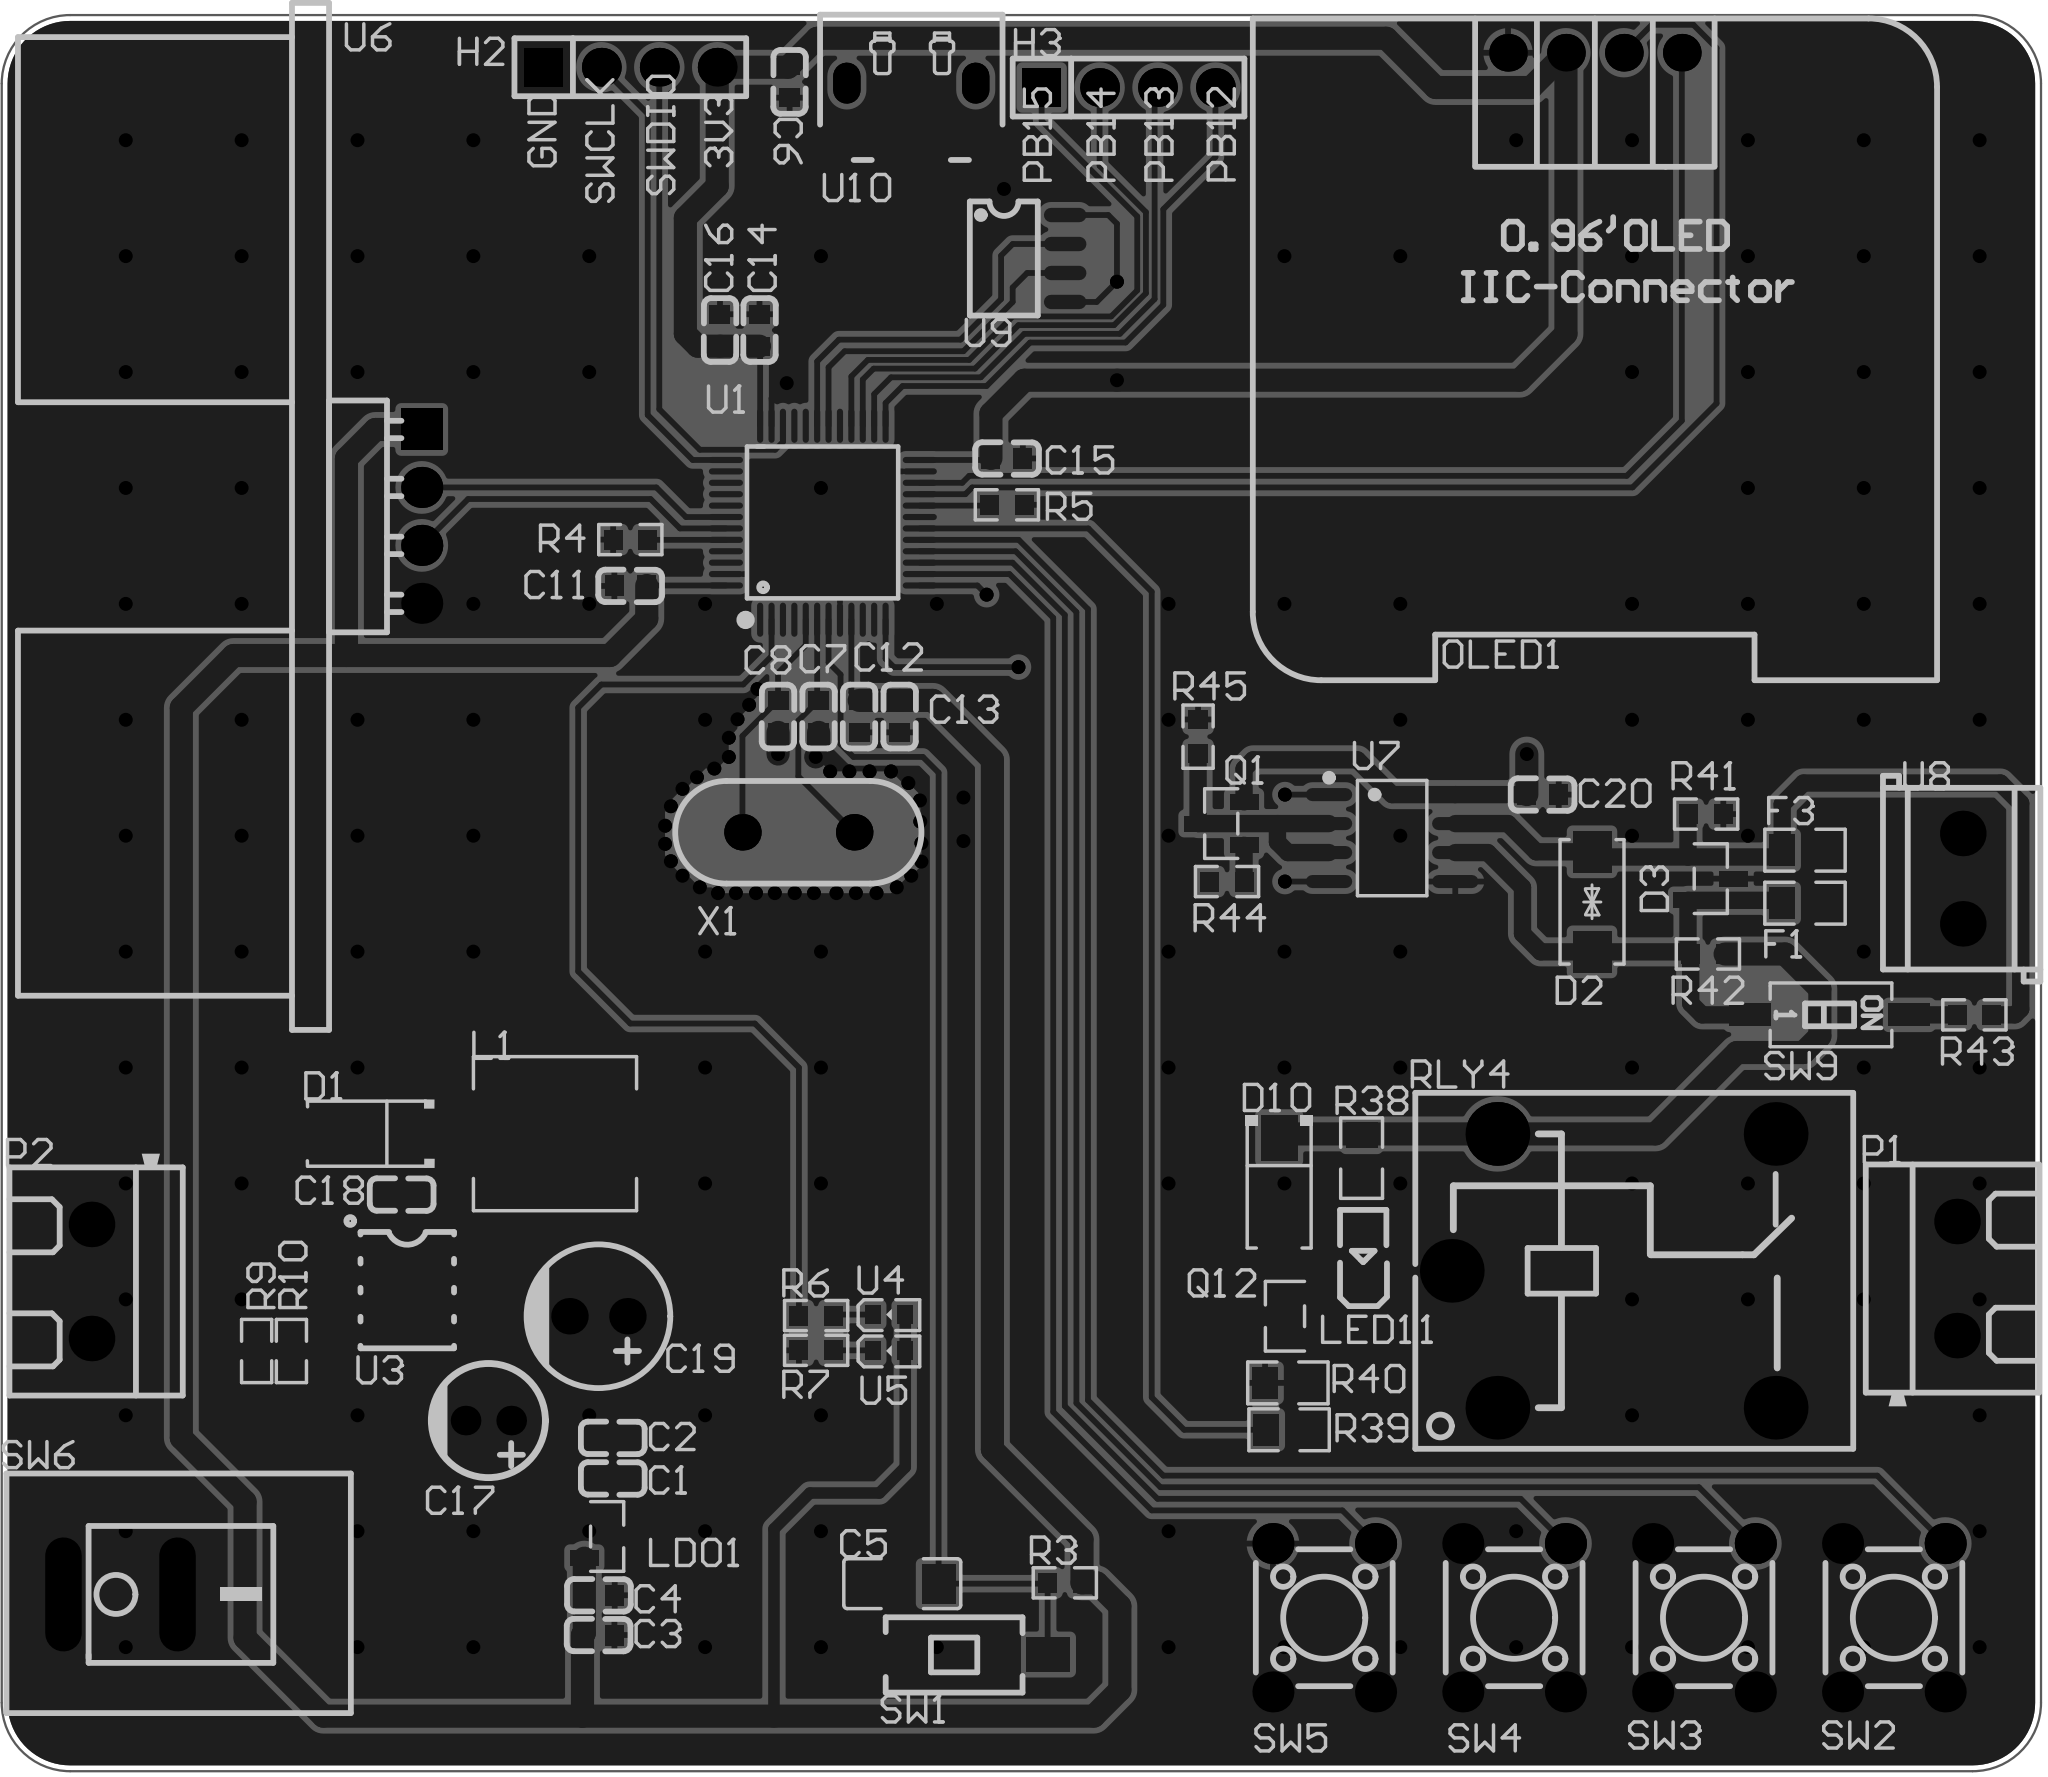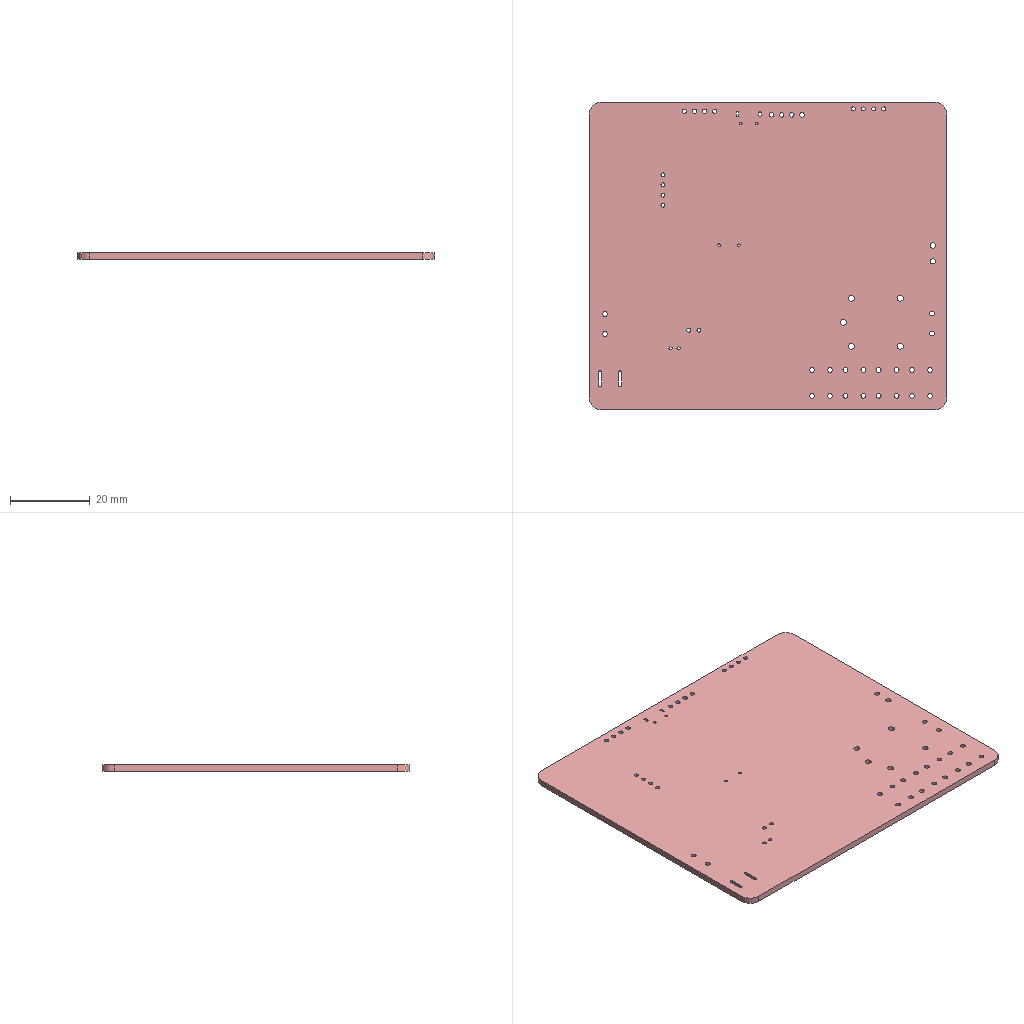Circuit board layout | Altium Designer | box 89.4 x 77 x 1.6 mm
Layer stack:
# Altium Designer layer stack of  (unit mm; dielectric type: 0 none, 1 core, 2 prepreg, 3 surface material)
index,name,kind,layer,copper_thickness_mm,dielectric_type,dielectric_thickness_mm,dielectric_material,dielectric_constant
0,Top Paste Mask Layer,other,,,,,,
1,Top Silkscreen Layer,other,,,,,,
2,Top Solder Mask Layer,dielectric,,,3,0.01,,3.3
3,Top Layer,copper,Top Layer,0.035,,,,
4,Dielectric1,dielectric,,,3,1.51,FR4,4.5
5,Bottom Layer,copper,Bottom Layer,0.035,,,,
6,Bottom Solder Mask Layer,dielectric,,,3,0.01,,3.3
7,Bottom Silkscreen Layer,other,,,,,,
8,Bottom Paste Mask Layer,other,,,,,,
# drill layer pairs: low layer,high layer
drill_pair,Top Layer,Bottom Layer
Part placement:
Designator,Comment,Layer,Footprint,Center-X(mm),Center-Y(mm),Rotation
C1,10uF,TopLayer,C0603,111.252,94.742,0
C2,100nF,TopLayer,C0603,111.252,96.52,0
C3,100nF,TopLayer,C0603,110.617,87.884,180
C4,10uF,TopLayer,C0603,110.63,89.626,180
C5,100uF,TopLayer,C1206,123.938,90.134,0
C6,100nF,TopLayer,C0603,118.999,155.956,90
C7,20pF,TopLayer,C0603,120.269,128.143,90
C8,20pF,TopLayer,C0603,118.491,128.143,90
C11,100nF,TopLayer,C0603,112.014,133.858,0
C12,100nF,TopLayer,C0603,122.047,128.143,90
C13,100nF,TopLayer,C0603,123.825,128.143,90
C14,100nF,TopLayer,C0603,117.678,145.067,270
C15,100nF,TopLayer,C0603,128.524,139.446,180
C16,4.7nF,TopLayer,C0603,115.946,145.067,270
C17,10uF,TopLayer,CAP-TH_BD5.0-P2.00-D0.8-FD,105.791,97.282,180
C18,10nF,TopLayer,C0603,101.981,107.188,180
C19,220uF,TopLayer,CAP-TH_BD6.3-P2.50-D1.0-FD,110.617,101.854,180
C20,100nF,TopLayer,C0603,152.019,124.714,0
D1,B340A,TopLayer,SMA_L4.3-W2.6-LS5.1-RD,100.457,109.855,180
D2,SMAJ7.0CA,TopLayer,SMA_L4.5-W2.7-LS5.1-BI,154.178,120.015,270
D3,SM712,TopLayer,SOT-23-3_L2.9-W1.3-P1.90-LS2.4-BR,159.385,121.031,180
D10,1N4007,TopLayer,SMA_L4.3-W2.5-LS5.0-RD,140.462,107.569,270
F1,0R,TopLayer,R0805,163.516,119.956,0
F3,0R,TopLayer,R0805,163.516,122.279,0
H2,,TopLayer,HDR-TH_4P-P2.54-V-M,112.014,156.591,0
L1,15uH,TopLayer,IND-SMD_L7.0-W6.6_FXL0630,108.712,109.855,0
LDO1,SC662K-3.3V,TopLayer,SOT-23-3_L2.9-W1.3-P1.90-LS2.4-BR,110.998,92.202,180
LED11,NCD0805R1,TopLayer,LED0805-R-RD,144.145,104.521,90
OLED1,,TopLayer,0.96OLED_4P,154.305,157.226,0
P1,KF301-2P terminal block,TopLayer,CONN-TH_XY301V-A-5.0-2P,170.18,103.505,270
P2,KF301-2P terminal block,TopLayer,CONN-TH_XY301V-A-5.0-2P,88.392,103.378,90
Q1,S8550-2TY,TopLayer,SOT-23-3_L2.9-W1.3-P0.95-LS2.4-BR,137.922,123.444,0
Q12,S8050 J3Y(RANGE:200-350),TopLayer,SOT-23-3_L3.0-W1.7-P0.95-LS2.9-BR,140.716,101.854,0
R3,1kΩ,TopLayer,R0603,131.064,90.17,0
R4,10kΩ,TopLayer,R0603,112.014,135.89,0
R5,10kΩ,TopLayer,R0603,128.524,137.414,180
R6,510Ω,TopLayer,R0603,120.16,101.884,180
R7,510Ω,TopLayer,R0603,120.16,100.36,180
R9,10kΩ,TopLayer,R0603,95.631,100.33,90
R10,3.24kΩ,TopLayer,R0603,97.155,100.33,90
R38,1.5kΩ,TopLayer,R0805,144.076,108.781,90
R39,1kΩ,TopLayer,R0805,140.896,96.878,0
R40,10kΩ,TopLayer,R0805,140.843,98.933,0
R41,3.3K,TopLayer,R0603,159.18,123.862,180
R42,3.3K,TopLayer,R0603,159.258,117.729,0
R43,120R,TopLayer,R0603,170.942,115.062,0
R44,4.7K,TopLayer,R0603,138.176,120.904,0
R45,10K,TopLayer,R0603,136.906,127.254,90
RLY4,SRD-05VDC-SL-C,TopLayer,RELAY-TH_SRD-XXVDC-XL-C,155.129,103.844,0
SW1,TS-1101-C-W,TopLayer,SW-SMD_L6.0-W3.3-LS8.0,126.347,87.028,0
SW2,,TopLayer,SW-TH_4P-L6.0-W6.0-P4.50-LS6.5,167.413,88.641,270
SW3,,TopLayer,SW-TH_4P-L6.0-W6.0-P4.50-LS6.5,159.088,88.641,270
SW4,,TopLayer,SW-TH_4P-L6.0-W6.0-P4.50-LS6.5,150.763,88.641,270
SW5,,TopLayer,SW-TH_4P-L6.0-W6.0-P4.50-LS6.5,142.438,88.641,270
U9,CH340N,TopLayer,SOP-8_L4.9-W3.9-P1.27-LS6.0-BL,128.397,148.209,270
U10,micro-B USB socket,TopLayer,MICRO-USB_C9900039549,124.333,154.433,180
SW9,ZX-1.27BM-1PSMD,TopLayer,SW-SMD_L5.4-W2.8-LS8.2,164.592,115.062,270
U1,STM32F103C8T6,TopLayer,LQFP-48_L7.0-W7.0-P0.50-LS9.0-BL,120.456,136.629,0
U3,TPS5430DDAR,TopLayer,ESOP-8_L4.9-W3.9-P1.27-LS6.0-TL-EP,102.235,102.997,0
U4,42-51/GHC-YW2X2K/3T,TopLayer,LED-SMD_L1.6-W0.8-FD_GREEN-1,123.353,101.928,180
U5,42-51/GHC-YW2X2K/3T,TopLayer,LED-SMD_L1.6-W0.8-FD_GREEN-1,123.353,100.336,180
U6,HC-SR04,TopLayer,TH_HC-SR04V,102.87,136.906,270
U7,MAX485ESA,TopLayer,SOP-8_L5.0-W4.0-P1.27-LS6.0-BL,145.415,122.809,270
U8,KF396-3.96-2P,TopLayer,CONN-TH_P3.96_KF396-3.96-2P,170.434,121.031,90
X1,8MHz,TopLayer,OSC-TH_L10.0-W4.5-P5.00,119.38,123.063,90
SW6,KCD11-2P-R,TopLayer,SW-TH_2P-L15.0-W10.5-P5.00_KCD11-2P-R,89.662,89.662,0
H3,,TopLayer,HDR-TH_4P-P2.54-V-M,133.858,155.702,0
Pad and via stacks:
# Altium Designer via and pad stacks of  (unit mm). Each distinct definition once, with the count of objects using it.
# via: kind,start_layer,end_layer,hole_mm,diameter_mm,mode(0 simple;1 top-mid-bottom;2 full stack),diameter_per_layer,count,example_net
# pad: kind,layer,hole_mm,hole_type(0 round;1 square;2 slot),plating,top_size,top_shape(1 round;2 rect;3 octagon;9 rounded rect),mid_size,bottom_size,mode,footprint,size_per_layer,count,example
pad,Top Layer,0,0,plated,0.8x0.9,2,0.8x0.9,0.8x0.9,0,C0603,,30,C1.2
pad,Top Layer,0,0,plated,1.485x1.728,2,1.485x1.728,1.485x1.728,0,C1206,,2,C5.2
pad,Top Layer,0,0,plated,2x2,2,2x2,2x2,0,SMA_L4.3-W2.6-LS5.1-RD,,2,D1.1
pad,Top Layer,0,0,plated,1.8x1.7,2,1.8x1.7,1.8x1.7,0,SMA_L4.5-W2.7-LS5.1-BI,,2,D2.1
pad,Top Layer,0,0,plated,1.25x0.7,2,1.25x0.7,1.25x0.7,0,SOT-23-3_L2.9-W1.3-P1.90-LS2.4-BR,,6,D3.1
pad,Top Layer,0,0,plated,2x1.593,2,2x1.593,2x1.593,0,SMA_L4.3-W2.5-LS5.0-RD,,2,D10.2
pad,Top Layer,0,0,plated,1.133x1.377,2,1.133x1.377,1.133x1.377,0,R0805,,10,F1.2
pad,Top Layer,0,0,plated,2.424x3.62,2,2.424x3.62,2.424x3.62,0,IND-SMD_L7.0-W6.6_FXL0630,,2,L1.1
pad,Top Layer,0,0,plated,1x1.399,2,1x1.399,1x1.399,0,LED0805-R-RD,,2,LED11.2
pad,Top Layer,0,0,plated,1.25x0.7,2,1.25x0.7,1.25x0.7,0,SOT-23-3_L2.9-W1.3-P0.95-LS2.4-BR,,3,Q1.1
pad,Top Layer,0,0,plated,1.038x0.532,2,1.038x0.532,1.038x0.532,0,SOT-23-3_L3.0-W1.7-P0.95-LS2.9-BR,,3,Q12.1
pad,Top Layer,0,0,plated,0.8065x0.864,2,0.8065x0.864,0.8065x0.864,0,R0603,,24,R3.2
pad,Top Layer,0,0,plated,1.9x1.5,2,1.9x1.5,1.9x1.5,0,SW-SMD_L6.0-W3.3-LS8.0,,2,SW1.1
pad,Top Layer,0,0,plated,0.63x1.865,1,0.63x1.865,0.63x1.865,0,SOP-8_L4.9-W3.9-P1.27-LS6.0-BL,,8,U9.1
pad,Top Layer,0,0,plated,1.4x1.25,2,1.4x1.25,1.4x1.25,0,MICRO-USB_C9900039549,,2,U10.7
pad,Top Layer,0,0,plated,0.4x1.85,2,0.4x1.85,0.4x1.85,0,MICRO-USB_C9900039549,,5,U10.5
pad,Top Layer,0,0,plated,1x1.8,2,1x1.8,1x1.8,0,SW-SMD_L5.4-W2.8-LS8.2,,2,SW9.2
pad,Top Layer,0,0,plated,0.27x1.5,1,0.27x1.5,0.27x1.5,0,LQFP-48_L7.0-W7.0-P0.50-LS9.0-BL,,24,U1.1
pad,Top Layer,0,0,plated,1.5x0.27,1,1.5x0.27,1.5x0.27,0,LQFP-48_L7.0-W7.0-P0.50-LS9.0-BL,,24,U1.13
pad,Top Layer,0,0,plated,1.3x0.6,2,1.3x0.6,1.3x0.6,0,ESOP-8_L4.9-W3.9-P1.27-LS6.0-TL-EP,,8,U3.1
pad,Top Layer,0,0,plated,2.5x3.5,2,2.5x3.5,2.5x3.5,0,ESOP-8_L4.9-W3.9-P1.27-LS6.0-TL-EP,,1,U3.9
pad,Top Layer,0,0,plated,0.8x0.7,2,0.8x0.7,0.8x0.7,0,LED-SMD_L1.6-W0.8-FD_GREEN-1,,4,U4.1
pad,Top Layer,0,0,plated,0.574x2.035,1,0.574x2.035,0.574x2.035,0,SOP-8_L5.0-W4.0-P1.27-LS6.0-BL,,8,U7.1
pad,Multi-Layer,0.8,0,plated,1.3x1.3,1,1.3x1.3,1.3x1.3,0,CAP-TH_BD5.0-P2.00-D0.8-FD,,2,C17.1
pad,Multi-Layer,1,0,plated,1.6x1.6,1,1.6x1.6,1.6x1.6,0,CAP-TH_BD6.3-P2.50-D1.0-FD,,2,C19.1
pad,Multi-Layer,1.1,0,plated,1.7x1.7,2,1.7x1.7,1.7x1.7,0,HDR-TH_4P-P2.54-V-M,,2,H2.1
pad,Multi-Layer,1.1,0,plated,1.7x1.7,1,1.7x1.7,1.7x1.7,0,HDR-TH_4P-P2.54-V-M,,6,H2.2
pad,Multi-Layer,1,0,plated,1.65x1.65,1,1.65x1.65,1.65x1.65,0,0.96OLED_4P,,4,OLED1.4
pad,Multi-Layer,1.2,0,plated,2x2,1,2x2,2x2,0,CONN-TH_XY301V-A-5.0-2P,,4,P1.1
pad,Multi-Layer,1.524,0,plated,2.794x2.794,1,2.794x2.794,2.794x2.794,0,RELAY-TH_SRD-XXVDC-XL-C,,5,RLY4.2
pad,Multi-Layer,1.2,0,plated,1.8x1.8,1,1.8x1.8,1.8x1.8,0,SW-TH_4P-L6.0-W6.0-P4.50-LS6.5,,16,SW2.1
pad,Multi-Layer,0.6,2,plated,1.8x1.2,1,1.8x1.2,1.8x1.2,0,MICRO-USB_C9900039549,,2,U10.7
pad,Multi-Layer,1.001,0,plated,1.8x1.8,1,1.8x1.8,1.8x1.8,0,TH_HC-SR04V,,3,U6.4
pad,Multi-Layer,1.001,0,plated,1.8x1.8,2,1.8x1.8,1.8x1.8,0,TH_HC-SR04V,,1,U6.1
pad,Multi-Layer,1.3,0,plated,2x2,1,2x2,2x2,0,CONN-TH_P3.96_KF396-3.96-2P,,2,U8.1
pad,Multi-Layer,0.7,0,plated,1.6x1.6,1,1.6x1.6,1.6x1.6,0,OSC-TH_L10.0-W4.5-P5.00,,2,X1.2
pad,Multi-Layer,0.8,2,plated,1.6x5,1,1.6x5,1.6x5,0,SW-TH_2P-L15.0-W10.5-P5.00_KCD11-2P-R,,2,SW6.1
via,Top Layer,Bottom Layer,0.3048,0.61,0,,176,3V3
via,Top Layer,Bottom Layer,0.3048,0.6096,0,,7,PA2
Copper pours:
name,layer,net,type(0 solid;1 hatched;2 none)
Top Layer-GND,Top Layer,GND,0
Bottom Layer-GND,Bottom Layer,GND,0